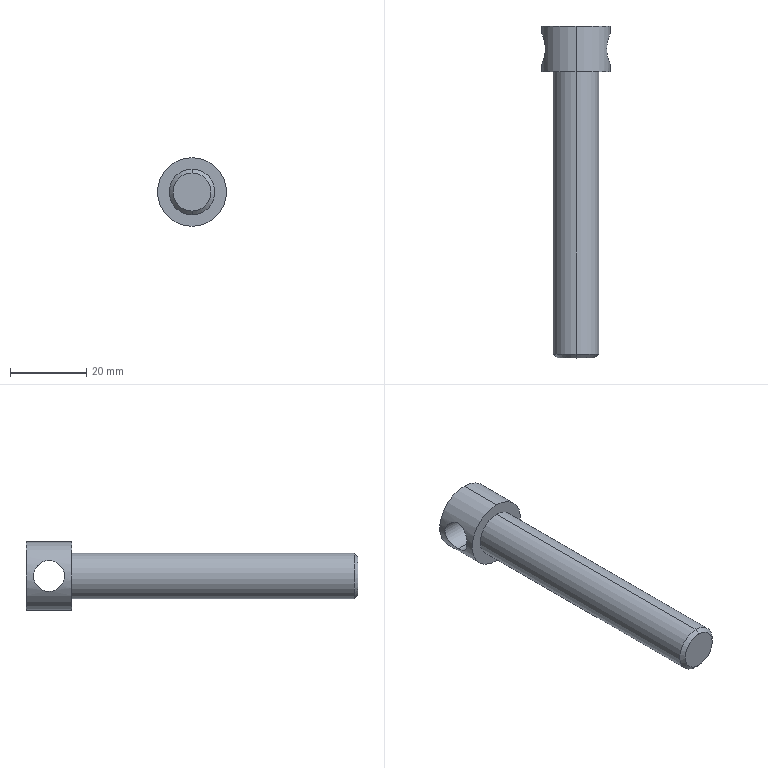Part | SolidWorks | features BaseBody 1 | 1 solid | 11 faces | box 18 x 87 x 18 mm | volume 10615 mm3 | cylinder 6 | plane 3 | cone 2 | commonest cylinder face diameters 8.1 x2 12 x2 18 x2
STEP:
#1=CARTESIAN_POINT('',(0.,-75.,-5.));
#2=VERTEX_POINT('',#1);
#3=CARTESIAN_POINT('',(0.,-75.,5.));
#4=VERTEX_POINT('',#3);
#5=CARTESIAN_POINT('',(0.,-75.,0.));
#6=DIRECTION('',(0.,-1.,0.));
#7=DIRECTION('',(0.,0.,-1.));
#8=AXIS2_PLACEMENT_3D('',#5,#6,#7);
#9=CIRCLE('',#8,5.);
#10=EDGE_CURVE('',#2,#4,#9,.T.);
#11=ORIENTED_EDGE('',*,*,#10,.F.);
#12=CARTESIAN_POINT('',(0.,-74.,-6.));
#13=VERTEX_POINT('',#12);
#14=CARTESIAN_POINT('',(0.,-75.,-5.));
#15=DIRECTION('',(0.,0.7071,-0.7071));
#16=VECTOR('',#15,1000.);
#17=LINE('',#14,#16);
#18=EDGE_CURVE('',#2,#13,#17,.T.);
#19=ORIENTED_EDGE('',*,*,#18,.T.);
#20=CARTESIAN_POINT('',(0.,-74.,6.));
#21=VERTEX_POINT('',#20);
#22=CARTESIAN_POINT('',(0.,-74.,0.));
#23=DIRECTION('',(0.,1.,0.));
#24=DIRECTION('',(0.,0.,-1.));
#25=AXIS2_PLACEMENT_3D('',#22,#23,#24);
#26=CIRCLE('',#25,6.);
#27=EDGE_CURVE('',#21,#13,#26,.T.);
#28=ORIENTED_EDGE('',*,*,#27,.F.);
#29=CARTESIAN_POINT('',(0.,-75.,5.));
#30=DIRECTION('',(0.,0.7071,0.7071));
#31=VECTOR('',#30,1000.);
#32=LINE('',#29,#31);
#33=EDGE_CURVE('',#4,#21,#32,.T.);
#34=ORIENTED_EDGE('',*,*,#33,.F.);
#35=EDGE_LOOP('',(#11,#19,#28,#34));
#36=FACE_OUTER_BOUND('',#35,.T.);
#37=CARTESIAN_POINT('',(0.,-75.,0.));
#38=DIRECTION('',(0.,1.,0.));
#39=DIRECTION('',(0.,0.,1.));
#40=AXIS2_PLACEMENT_3D('',#37,#38,#39);
#41=CONICAL_SURFACE('',#40,5.,0.7854);
#42=ADVANCED_FACE('',(#36),#41,.T.);
#43=CARTESIAN_POINT('',(-8.037,6.,4.05));
#44=VERTEX_POINT('',#43);
#45=CARTESIAN_POINT('',(-8.037,6.,-4.05));
#46=VERTEX_POINT('',#45);
#47=CARTESIAN_POINT('',(-8.037,6.,4.05));
#48=CARTESIAN_POINT('',(-8.037,5.729,4.05));
#49=CARTESIAN_POINT('',(-8.051,5.462,4.023));
#50=CARTESIAN_POINT('',(-8.103,4.94,3.918));
#51=CARTESIAN_POINT('',(-8.141,4.682,3.839));
#52=CARTESIAN_POINT('',(-8.234,4.194,3.634));
#53=CARTESIAN_POINT('',(-8.289,3.963,3.51));
#54=CARTESIAN_POINT('',(-8.407,3.525,3.217));
#55=CARTESIAN_POINT('',(-8.47,3.322,3.049));
#56=CARTESIAN_POINT('',(-8.594,2.953,2.681));
#57=CARTESIAN_POINT('',(-8.655,2.786,2.478));
#58=CARTESIAN_POINT('',(-8.769,2.491,2.04));
#59=CARTESIAN_POINT('',(-8.82,2.367,1.809));
#60=CARTESIAN_POINT('',(-8.906,2.163,1.323));
#61=CARTESIAN_POINT('',(-8.941,2.083,1.064));
#62=CARTESIAN_POINT('',(-8.988,1.977,0.5394));
#63=CARTESIAN_POINT('',(-9.,1.95,0.274));
#64=CARTESIAN_POINT('',(-9.,1.95,-0.2628));
#65=CARTESIAN_POINT('',(-8.988,1.977,-0.5348));
#66=CARTESIAN_POINT('',(-8.941,2.082,-1.058));
#67=CARTESIAN_POINT('',(-8.907,2.16,-1.314));
#68=CARTESIAN_POINT('',(-8.82,2.366,-1.807));
#69=CARTESIAN_POINT('',(-8.769,2.491,-2.038));
#70=CARTESIAN_POINT('',(-8.656,2.783,-2.474));
#71=CARTESIAN_POINT('',(-8.594,2.952,-2.68));
#72=CARTESIAN_POINT('',(-8.47,3.321,-3.049));
#73=CARTESIAN_POINT('',(-8.408,3.522,-3.214));
#74=CARTESIAN_POINT('',(-8.29,3.959,-3.508));
#75=CARTESIAN_POINT('',(-8.235,4.193,-3.634));
#76=CARTESIAN_POINT('',(-8.142,4.677,-3.837));
#77=CARTESIAN_POINT('',(-8.104,4.931,-3.916));
#78=CARTESIAN_POINT('',(-8.051,5.46,-4.023));
#79=CARTESIAN_POINT('',(-8.037,5.728,-4.05));
#80=CARTESIAN_POINT('',(-8.037,6.,-4.05));
#81=B_SPLINE_CURVE_WITH_KNOTS('',3,(#47,#48,#49,#50,#51,#52,#53,#54,#55,#56,#57,#58,#59,#60,#61,#62,#63,#64,#65,#66,#67,#68,#69,#70,#71,#72,#73,#74,#75,#76,#77,#78,#79,#80),.UNSPECIFIED.,.F.,.F.,(4,2,2,2,2,2,2,2,2,2,2,2,2,2,2,2,4),(0.,0.0008018,0.001604,0.002406,0.003207,0.004009,0.004811,0.005613,0.006415,0.007217,0.008018,0.00882,0.009622,0.01042,0.01123,0.01203,0.01283),.UNSPECIFIED.);
#82=EDGE_CURVE('',#44,#46,#81,.T.);
#83=ORIENTED_EDGE('',*,*,#82,.F.);
#84=CARTESIAN_POINT('',(8.037,6.,4.05));
#85=VERTEX_POINT('',#84);
#86=CARTESIAN_POINT('',(-9.,6.,4.05));
#87=DIRECTION('',(1.,0.,0.));
#88=VECTOR('',#87,1000.);
#89=LINE('',#86,#88);
#90=EDGE_CURVE('',#44,#85,#89,.T.);
#91=ORIENTED_EDGE('',*,*,#90,.T.);
#92=CARTESIAN_POINT('',(8.037,6.,-4.05));
#93=VERTEX_POINT('',#92);
#94=CARTESIAN_POINT('',(8.037,6.,-4.05));
#95=CARTESIAN_POINT('',(8.037,5.729,-4.05));
#96=CARTESIAN_POINT('',(8.051,5.462,-4.023));
#97=CARTESIAN_POINT('',(8.103,4.94,-3.918));
#98=CARTESIAN_POINT('',(8.141,4.682,-3.839));
#99=CARTESIAN_POINT('',(8.234,4.194,-3.634));
#100=CARTESIAN_POINT('',(8.289,3.963,-3.51));
#101=CARTESIAN_POINT('',(8.407,3.525,-3.217));
#102=CARTESIAN_POINT('',(8.47,3.322,-3.049));
#103=CARTESIAN_POINT('',(8.594,2.953,-2.681));
#104=CARTESIAN_POINT('',(8.655,2.786,-2.478));
#105=CARTESIAN_POINT('',(8.769,2.491,-2.04));
#106=CARTESIAN_POINT('',(8.82,2.367,-1.809));
#107=CARTESIAN_POINT('',(8.906,2.163,-1.323));
#108=CARTESIAN_POINT('',(8.941,2.083,-1.064));
#109=CARTESIAN_POINT('',(8.988,1.977,-0.5394));
#110=CARTESIAN_POINT('',(9.,1.95,-0.274));
#111=CARTESIAN_POINT('',(9.,1.95,0.2628));
#112=CARTESIAN_POINT('',(8.988,1.977,0.5348));
#113=CARTESIAN_POINT('',(8.941,2.082,1.058));
#114=CARTESIAN_POINT('',(8.907,2.16,1.314));
#115=CARTESIAN_POINT('',(8.82,2.366,1.807));
#116=CARTESIAN_POINT('',(8.769,2.491,2.038));
#117=CARTESIAN_POINT('',(8.656,2.783,2.474));
#118=CARTESIAN_POINT('',(8.594,2.952,2.68));
#119=CARTESIAN_POINT('',(8.47,3.321,3.049));
#120=CARTESIAN_POINT('',(8.408,3.522,3.214));
#121=CARTESIAN_POINT('',(8.29,3.959,3.508));
#122=CARTESIAN_POINT('',(8.235,4.193,3.634));
#123=CARTESIAN_POINT('',(8.142,4.677,3.837));
#124=CARTESIAN_POINT('',(8.104,4.931,3.916));
#125=CARTESIAN_POINT('',(8.051,5.46,4.023));
#126=CARTESIAN_POINT('',(8.037,5.728,4.05));
#127=CARTESIAN_POINT('',(8.037,6.,4.05));
#128=B_SPLINE_CURVE_WITH_KNOTS('',3,(#94,#95,#96,#97,#98,#99,#100,#101,#102,#103,#104,#105,#106,#107,#108,#109,#110,#111,#112,#113,#114,#115,#116,#117,#118,#119,#120,#121,#122,#123,#124,#125,#126,#127),.UNSPECIFIED.,.F.,.F.,(4,2,2,2,2,2,2,2,2,2,2,2,2,2,2,2,4),(0.,0.0008018,0.001604,0.002406,0.003207,0.004009,0.004811,0.005613,0.006415,0.007217,0.008018,0.00882,0.009622,0.01042,0.01123,0.01203,0.01283),.UNSPECIFIED.);
#129=EDGE_CURVE('',#93,#85,#128,.T.);
#130=ORIENTED_EDGE('',*,*,#129,.F.);
#131=CARTESIAN_POINT('',(-9.,6.,-4.05));
#132=DIRECTION('',(1.,0.,0.));
#133=VECTOR('',#132,1000.);
#134=LINE('',#131,#133);
#135=EDGE_CURVE('',#46,#93,#134,.T.);
#136=ORIENTED_EDGE('',*,*,#135,.F.);
#137=EDGE_LOOP('',(#83,#91,#130,#136));
#138=FACE_OUTER_BOUND('',#137,.T.);
#139=CARTESIAN_POINT('',(-9.,6.,0.));
#140=DIRECTION('',(1.,0.,0.));
#141=DIRECTION('',(0.,0.,-1.));
#142=AXIS2_PLACEMENT_3D('',#139,#140,#141);
#143=CYLINDRICAL_SURFACE('',#142,4.05);
#144=ADVANCED_FACE('',(#138),#143,.F.);
#145=ORIENTED_EDGE('',*,*,#27,.T.);
#146=CARTESIAN_POINT('',(0.,0.,-6.));
#147=VERTEX_POINT('',#146);
#148=CARTESIAN_POINT('',(0.,-75.,-6.));
#149=DIRECTION('',(0.,1.,0.));
#150=VECTOR('',#149,1000.);
#151=LINE('',#148,#150);
#152=EDGE_CURVE('',#13,#147,#151,.T.);
#153=ORIENTED_EDGE('',*,*,#152,.T.);
#154=CARTESIAN_POINT('',(0.,0.,6.));
#155=VERTEX_POINT('',#154);
#156=CARTESIAN_POINT('',(0.,0.,0.));
#157=DIRECTION('',(0.,-1.,0.));
#158=DIRECTION('',(0.,0.,1.));
#159=AXIS2_PLACEMENT_3D('',#156,#157,#158);
#160=CIRCLE('',#159,6.);
#161=EDGE_CURVE('',#147,#155,#160,.T.);
#162=ORIENTED_EDGE('',*,*,#161,.T.);
#163=CARTESIAN_POINT('',(0.,-75.,6.));
#164=DIRECTION('',(0.,1.,0.));
#165=VECTOR('',#164,1000.);
#166=LINE('',#163,#165);
#167=EDGE_CURVE('',#21,#155,#166,.T.);
#168=ORIENTED_EDGE('',*,*,#167,.F.);
#169=EDGE_LOOP('',(#145,#153,#162,#168));
#170=FACE_OUTER_BOUND('',#169,.T.);
#171=CARTESIAN_POINT('',(0.,-75.,0.));
#172=DIRECTION('',(0.,1.,0.));
#173=DIRECTION('',(0.,0.,1.));
#174=AXIS2_PLACEMENT_3D('',#171,#172,#173);
#175=CYLINDRICAL_SURFACE('',#174,6.);
#176=ADVANCED_FACE('',(#170),#175,.T.);
#177=ORIENTED_EDGE('',*,*,#129,.T.);
#178=CARTESIAN_POINT('',(8.037,6.,4.05));
#179=CARTESIAN_POINT('',(8.037,6.271,4.05));
#180=CARTESIAN_POINT('',(8.051,6.538,4.023));
#181=CARTESIAN_POINT('',(8.103,7.06,3.918));
#182=CARTESIAN_POINT('',(8.141,7.318,3.839));
#183=CARTESIAN_POINT('',(8.234,7.806,3.634));
#184=CARTESIAN_POINT('',(8.289,8.037,3.51));
#185=CARTESIAN_POINT('',(8.407,8.475,3.217));
#186=CARTESIAN_POINT('',(8.47,8.678,3.049));
#187=CARTESIAN_POINT('',(8.594,9.047,2.681));
#188=CARTESIAN_POINT('',(8.655,9.214,2.478));
#189=CARTESIAN_POINT('',(8.769,9.509,2.04));
#190=CARTESIAN_POINT('',(8.82,9.633,1.809));
#191=CARTESIAN_POINT('',(8.906,9.837,1.323));
#192=CARTESIAN_POINT('',(8.941,9.917,1.064));
#193=CARTESIAN_POINT('',(8.988,10.023,0.5394));
#194=CARTESIAN_POINT('',(9.,10.05,0.274));
#195=CARTESIAN_POINT('',(9.,10.05,-0.2628));
#196=CARTESIAN_POINT('',(8.988,10.023,-0.5348));
#197=CARTESIAN_POINT('',(8.941,9.918,-1.058));
#198=CARTESIAN_POINT('',(8.907,9.84,-1.314));
#199=CARTESIAN_POINT('',(8.82,9.634,-1.807));
#200=CARTESIAN_POINT('',(8.769,9.509,-2.038));
#201=CARTESIAN_POINT('',(8.656,9.217,-2.474));
#202=CARTESIAN_POINT('',(8.594,9.048,-2.68));
#203=CARTESIAN_POINT('',(8.47,8.679,-3.049));
#204=CARTESIAN_POINT('',(8.408,8.478,-3.214));
#205=CARTESIAN_POINT('',(8.29,8.041,-3.508));
#206=CARTESIAN_POINT('',(8.235,7.807,-3.634));
#207=CARTESIAN_POINT('',(8.142,7.323,-3.837));
#208=CARTESIAN_POINT('',(8.104,7.069,-3.916));
#209=CARTESIAN_POINT('',(8.051,6.54,-4.023));
#210=CARTESIAN_POINT('',(8.037,6.271,-4.05));
#211=CARTESIAN_POINT('',(8.037,6.,-4.05));
#212=B_SPLINE_CURVE_WITH_KNOTS('',3,(#178,#179,#180,#181,#182,#183,#184,#185,#186,#187,#188,#189,#190,#191,#192,#193,#194,#195,#196,#197,#198,#199,#200,#201,#202,#203,#204,#205,#206,#207,#208,#209,#210,#211),.UNSPECIFIED.,.F.,.F.,(4,2,2,2,2,2,2,2,2,2,2,2,2,2,2,2,4),(0.01283,0.01363,0.01443,0.01523,0.01604,0.01684,0.01764,0.01844,0.01924,0.02004,0.02084,0.02165,0.02245,0.02325,0.02405,0.02485,0.02565),.UNSPECIFIED.);
#213=EDGE_CURVE('',#85,#93,#212,.T.);
#214=ORIENTED_EDGE('',*,*,#213,.T.);
#215=EDGE_LOOP('',(#177,#214));
#216=FACE_BOUND('',#215,.T.);
#217=CARTESIAN_POINT('',(0.,12.,9.));
#218=VERTEX_POINT('',#217);
#219=CARTESIAN_POINT('',(0.,12.,-9.));
#220=VERTEX_POINT('',#219);
#221=CARTESIAN_POINT('',(0.,12.,0.));
#222=DIRECTION('',(0.,1.,0.));
#223=DIRECTION('',(0.,0.,1.));
#224=AXIS2_PLACEMENT_3D('',#221,#222,#223);
#225=CIRCLE('',#224,9.);
#226=EDGE_CURVE('',#218,#220,#225,.T.);
#227=ORIENTED_EDGE('',*,*,#226,.F.);
#228=CARTESIAN_POINT('',(0.,0.,9.));
#229=VERTEX_POINT('',#228);
#230=CARTESIAN_POINT('',(0.,12.,9.));
#231=DIRECTION('',(0.,-1.,0.));
#232=VECTOR('',#231,1000.);
#233=LINE('',#230,#232);
#234=EDGE_CURVE('',#218,#229,#233,.T.);
#235=ORIENTED_EDGE('',*,*,#234,.T.);
#236=CARTESIAN_POINT('',(0.,0.,-9.));
#237=VERTEX_POINT('',#236);
#238=CARTESIAN_POINT('',(0.,0.,0.));
#239=DIRECTION('',(0.,1.,0.));
#240=DIRECTION('',(0.,0.,1.));
#241=AXIS2_PLACEMENT_3D('',#238,#239,#240);
#242=CIRCLE('',#241,9.);
#243=EDGE_CURVE('',#229,#237,#242,.T.);
#244=ORIENTED_EDGE('',*,*,#243,.T.);
#245=CARTESIAN_POINT('',(0.,12.,-9.));
#246=DIRECTION('',(0.,-1.,0.));
#247=VECTOR('',#246,1000.);
#248=LINE('',#245,#247);
#249=EDGE_CURVE('',#220,#237,#248,.T.);
#250=ORIENTED_EDGE('',*,*,#249,.F.);
#251=EDGE_LOOP('',(#227,#235,#244,#250));
#252=FACE_OUTER_BOUND('',#251,.T.);
#253=CARTESIAN_POINT('',(0.,12.,0.));
#254=DIRECTION('',(0.,-1.,0.));
#255=DIRECTION('',(0.,0.,-1.));
#256=AXIS2_PLACEMENT_3D('',#253,#254,#255);
#257=CYLINDRICAL_SURFACE('',#256,9.);
#258=ADVANCED_FACE('',(#216,#252),#257,.T.);
#259=CARTESIAN_POINT('',(0.,-75.,0.));
#260=DIRECTION('',(0.,-1.,0.));
#261=DIRECTION('',(0.,0.,-1.));
#262=AXIS2_PLACEMENT_3D('',#259,#260,#261);
#263=CIRCLE('',#262,5.);
#264=EDGE_CURVE('',#4,#2,#263,.T.);
#265=ORIENTED_EDGE('',*,*,#264,.T.);
#266=ORIENTED_EDGE('',*,*,#10,.T.);
#267=EDGE_LOOP('',(#265,#266));
#268=FACE_OUTER_BOUND('',#267,.T.);
#269=CARTESIAN_POINT('',(0.,-75.,0.));
#270=DIRECTION('',(0.,-1.,0.));
#271=DIRECTION('',(0.,0.,-1.));
#272=AXIS2_PLACEMENT_3D('',#269,#270,#271);
#273=PLANE('',#272);
#274=ADVANCED_FACE('',(#268),#273,.T.);
#275=CARTESIAN_POINT('',(0.,12.,0.));
#276=DIRECTION('',(0.,1.,0.));
#277=DIRECTION('',(0.,0.,1.));
#278=AXIS2_PLACEMENT_3D('',#275,#276,#277);
#279=CIRCLE('',#278,9.);
#280=EDGE_CURVE('',#220,#218,#279,.T.);
#281=ORIENTED_EDGE('',*,*,#280,.T.);
#282=ORIENTED_EDGE('',*,*,#226,.T.);
#283=EDGE_LOOP('',(#281,#282));
#284=FACE_OUTER_BOUND('',#283,.T.);
#285=CARTESIAN_POINT('',(0.,12.,0.));
#286=DIRECTION('',(0.,1.,0.));
#287=DIRECTION('',(1.,0.,0.));
#288=AXIS2_PLACEMENT_3D('',#285,#286,#287);
#289=PLANE('',#288);
#290=ADVANCED_FACE('',(#284),#289,.T.);
#291=CARTESIAN_POINT('',(0.,0.,0.));
#292=DIRECTION('',(0.,-1.,0.));
#293=DIRECTION('',(0.,0.,1.));
#294=AXIS2_PLACEMENT_3D('',#291,#292,#293);
#295=CIRCLE('',#294,6.);
#296=EDGE_CURVE('',#155,#147,#295,.T.);
#297=ORIENTED_EDGE('',*,*,#296,.F.);
#298=ORIENTED_EDGE('',*,*,#161,.F.);
#299=EDGE_LOOP('',(#297,#298));
#300=FACE_BOUND('',#299,.T.);
#301=CARTESIAN_POINT('',(0.,0.,0.));
#302=DIRECTION('',(0.,1.,0.));
#303=DIRECTION('',(0.,0.,1.));
#304=AXIS2_PLACEMENT_3D('',#301,#302,#303);
#305=CIRCLE('',#304,9.);
#306=EDGE_CURVE('',#237,#229,#305,.T.);
#307=ORIENTED_EDGE('',*,*,#306,.F.);
#308=ORIENTED_EDGE('',*,*,#243,.F.);
#309=EDGE_LOOP('',(#307,#308));
#310=FACE_OUTER_BOUND('',#309,.T.);
#311=CARTESIAN_POINT('',(0.,0.,0.));
#312=DIRECTION('',(0.,1.,0.));
#313=DIRECTION('',(1.,0.,0.));
#314=AXIS2_PLACEMENT_3D('',#311,#312,#313);
#315=PLANE('',#314);
#316=ADVANCED_FACE('',(#300,#310),#315,.F.);
#317=ORIENTED_EDGE('',*,*,#234,.F.);
#318=ORIENTED_EDGE('',*,*,#280,.F.);
#319=ORIENTED_EDGE('',*,*,#249,.T.);
#320=ORIENTED_EDGE('',*,*,#306,.T.);
#321=EDGE_LOOP('',(#317,#318,#319,#320));
#322=FACE_OUTER_BOUND('',#321,.T.);
#323=CARTESIAN_POINT('',(-8.037,6.,-4.05));
#324=CARTESIAN_POINT('',(-8.037,6.271,-4.05));
#325=CARTESIAN_POINT('',(-8.051,6.538,-4.023));
#326=CARTESIAN_POINT('',(-8.103,7.06,-3.918));
#327=CARTESIAN_POINT('',(-8.141,7.318,-3.839));
#328=CARTESIAN_POINT('',(-8.234,7.806,-3.634));
#329=CARTESIAN_POINT('',(-8.289,8.037,-3.51));
#330=CARTESIAN_POINT('',(-8.407,8.475,-3.217));
#331=CARTESIAN_POINT('',(-8.47,8.678,-3.049));
#332=CARTESIAN_POINT('',(-8.594,9.047,-2.681));
#333=CARTESIAN_POINT('',(-8.655,9.214,-2.478));
#334=CARTESIAN_POINT('',(-8.769,9.509,-2.04));
#335=CARTESIAN_POINT('',(-8.82,9.633,-1.809));
#336=CARTESIAN_POINT('',(-8.906,9.837,-1.323));
#337=CARTESIAN_POINT('',(-8.941,9.917,-1.064));
#338=CARTESIAN_POINT('',(-8.988,10.023,-0.5394));
#339=CARTESIAN_POINT('',(-9.,10.05,-0.274));
#340=CARTESIAN_POINT('',(-9.,10.05,0.2628));
#341=CARTESIAN_POINT('',(-8.988,10.023,0.5348));
#342=CARTESIAN_POINT('',(-8.941,9.918,1.058));
#343=CARTESIAN_POINT('',(-8.907,9.84,1.314));
#344=CARTESIAN_POINT('',(-8.82,9.634,1.807));
#345=CARTESIAN_POINT('',(-8.769,9.509,2.038));
#346=CARTESIAN_POINT('',(-8.656,9.217,2.474));
#347=CARTESIAN_POINT('',(-8.594,9.048,2.68));
#348=CARTESIAN_POINT('',(-8.47,8.679,3.049));
#349=CARTESIAN_POINT('',(-8.408,8.478,3.214));
#350=CARTESIAN_POINT('',(-8.29,8.041,3.508));
#351=CARTESIAN_POINT('',(-8.235,7.807,3.634));
#352=CARTESIAN_POINT('',(-8.142,7.323,3.837));
#353=CARTESIAN_POINT('',(-8.104,7.069,3.916));
#354=CARTESIAN_POINT('',(-8.051,6.54,4.023));
#355=CARTESIAN_POINT('',(-8.037,6.271,4.05));
#356=CARTESIAN_POINT('',(-8.037,6.,4.05));
#357=B_SPLINE_CURVE_WITH_KNOTS('',3,(#323,#324,#325,#326,#327,#328,#329,#330,#331,#332,#333,#334,#335,#336,#337,#338,#339,#340,#341,#342,#343,#344,#345,#346,#347,#348,#349,#350,#351,#352,#353,#354,#355,#356),.UNSPECIFIED.,.F.,.F.,(4,2,2,2,2,2,2,2,2,2,2,2,2,2,2,2,4),(0.01283,0.01363,0.01443,0.01523,0.01604,0.01684,0.01764,0.01844,0.01924,0.02004,0.02084,0.02165,0.02245,0.02325,0.02405,0.02485,0.02565),.UNSPECIFIED.);
#358=EDGE_CURVE('',#46,#44,#357,.T.);
#359=ORIENTED_EDGE('',*,*,#358,.T.);
#360=ORIENTED_EDGE('',*,*,#82,.T.);
#361=EDGE_LOOP('',(#359,#360));
#362=FACE_BOUND('',#361,.T.);
#363=CARTESIAN_POINT('',(0.,12.,0.));
#364=DIRECTION('',(0.,-1.,0.));
#365=DIRECTION('',(0.,0.,-1.));
#366=AXIS2_PLACEMENT_3D('',#363,#364,#365);
#367=CYLINDRICAL_SURFACE('',#366,9.);
#368=ADVANCED_FACE('',(#322,#362),#367,.T.);
#369=ORIENTED_EDGE('',*,*,#152,.F.);
#370=CARTESIAN_POINT('',(0.,-74.,0.));
#371=DIRECTION('',(0.,1.,0.));
#372=DIRECTION('',(0.,0.,-1.));
#373=AXIS2_PLACEMENT_3D('',#370,#371,#372);
#374=CIRCLE('',#373,6.);
#375=EDGE_CURVE('',#13,#21,#374,.T.);
#376=ORIENTED_EDGE('',*,*,#375,.T.);
#377=ORIENTED_EDGE('',*,*,#167,.T.);
#378=ORIENTED_EDGE('',*,*,#296,.T.);
#379=EDGE_LOOP('',(#369,#376,#377,#378));
#380=FACE_OUTER_BOUND('',#379,.T.);
#381=CARTESIAN_POINT('',(0.,-75.,0.));
#382=DIRECTION('',(0.,1.,0.));
#383=DIRECTION('',(0.,0.,1.));
#384=AXIS2_PLACEMENT_3D('',#381,#382,#383);
#385=CYLINDRICAL_SURFACE('',#384,6.);
#386=ADVANCED_FACE('',(#380),#385,.T.);
#387=ORIENTED_EDGE('',*,*,#90,.F.);
#388=ORIENTED_EDGE('',*,*,#358,.F.);
#389=ORIENTED_EDGE('',*,*,#135,.T.);
#390=ORIENTED_EDGE('',*,*,#213,.F.);
#391=EDGE_LOOP('',(#387,#388,#389,#390));
#392=FACE_OUTER_BOUND('',#391,.T.);
#393=CARTESIAN_POINT('',(-9.,6.,0.));
#394=DIRECTION('',(1.,0.,0.));
#395=DIRECTION('',(0.,0.,-1.));
#396=AXIS2_PLACEMENT_3D('',#393,#394,#395);
#397=CYLINDRICAL_SURFACE('',#396,4.05);
#398=ADVANCED_FACE('',(#392),#397,.F.);
#399=ORIENTED_EDGE('',*,*,#18,.F.);
#400=ORIENTED_EDGE('',*,*,#264,.F.);
#401=ORIENTED_EDGE('',*,*,#33,.T.);
#402=ORIENTED_EDGE('',*,*,#375,.F.);
#403=EDGE_LOOP('',(#399,#400,#401,#402));
#404=FACE_OUTER_BOUND('',#403,.T.);
#405=CARTESIAN_POINT('',(0.,-75.,0.));
#406=DIRECTION('',(0.,1.,0.));
#407=DIRECTION('',(0.,0.,1.));
#408=AXIS2_PLACEMENT_3D('',#405,#406,#407);
#409=CONICAL_SURFACE('',#408,5.,0.7854);
#410=ADVANCED_FACE('',(#404),#409,.T.);
#411=CLOSED_SHELL('',(#42,#144,#176,#258,#274,#290,#316,#368,#386,#398,#410));
#412=MANIFOLD_SOLID_BREP('',#411);
#413=CARTESIAN_POINT('',(0.,0.,0.));
#414=DIRECTION('',(0.,0.,1.));
#415=DIRECTION('',(1.,0.,0.));
#416=AXIS2_PLACEMENT_3D('',#413,#414,#415);
#417=(LENGTH_UNIT()NAMED_UNIT(*)SI_UNIT(.MILLI.,.METRE.));
#418=UNCERTAINTY_MEASURE_WITH_UNIT(LENGTH_MEASURE(0.00001),#417,'','');
#419=(NAMED_UNIT(*)PLANE_ANGLE_UNIT()SI_UNIT($,.RADIAN.));
#420=(NAMED_UNIT(*)SI_UNIT($,.STERADIAN.)SOLID_ANGLE_UNIT());
#421=(GEOMETRIC_REPRESENTATION_CONTEXT(3)GLOBAL_UNCERTAINTY_ASSIGNED_CONTEXT((#418))GLOBAL_UNIT_ASSIGNED_CONTEXT((#417,#419,#420))REPRESENTATION_CONTEXT('',''));
#422=ADVANCED_BREP_SHAPE_REPRESENTATION('',(#412,#416),#421);